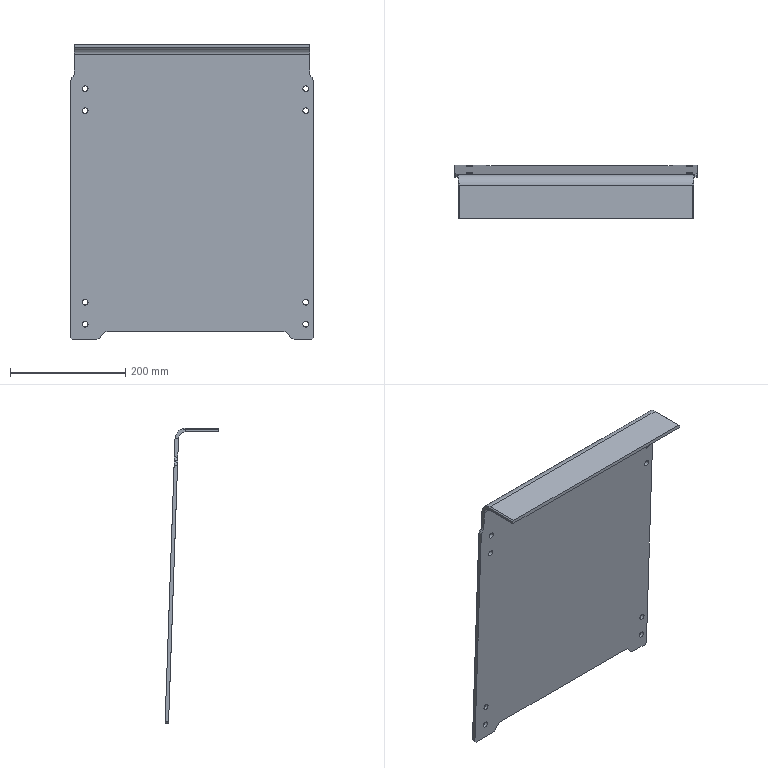Part | SolidWorks | features Cut 1, FlatPattern 1, SM3dBend 1, SMBaseFlange 1, SheetMetal 1 | 1 solid | 50 faces | box 420 x 93.297 x 511.152 mm | volume 1409801 mm3 | cylinder 26 | plane 24 | commonest cylinder face diameters 10 x16 20 x8 24 x1 36 x1